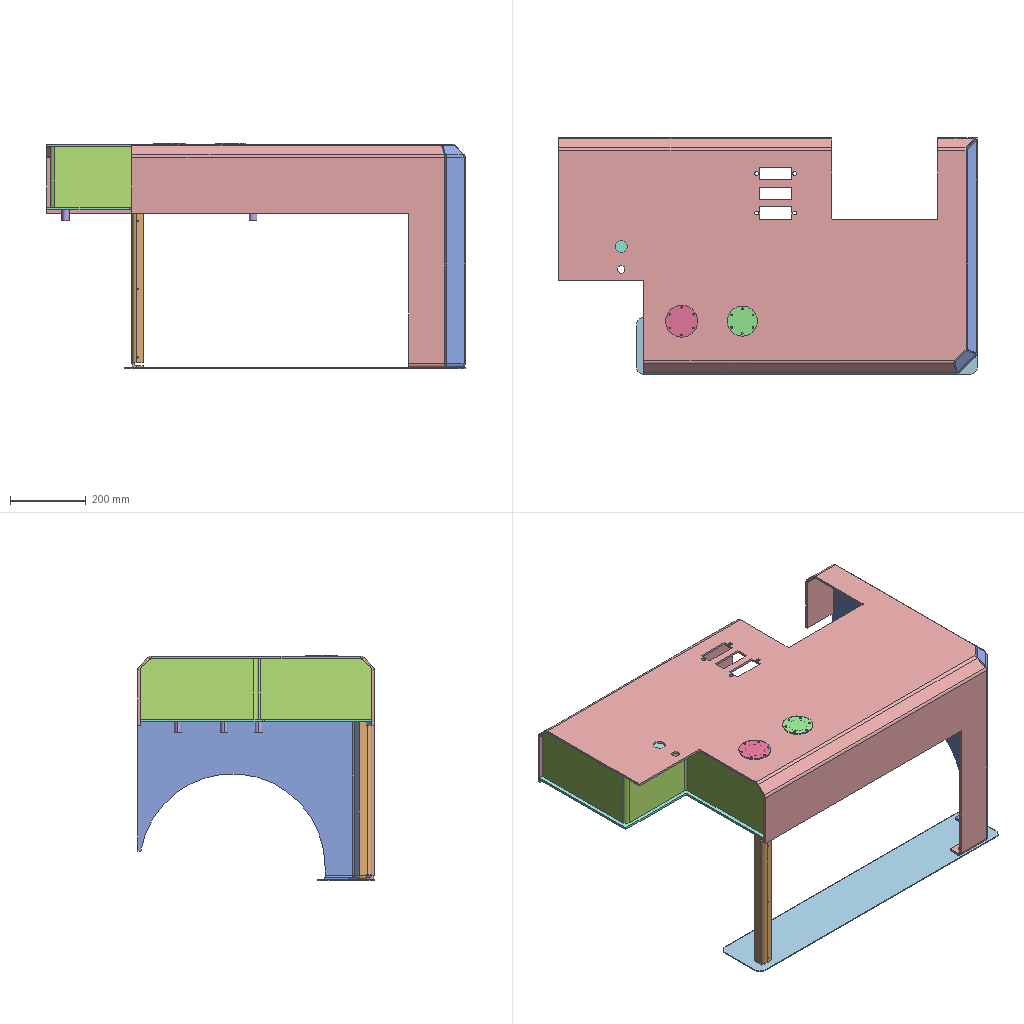Assembly | SolidWorks | 10 different items | 12 placed | box 1106 x 624 x 595 mm
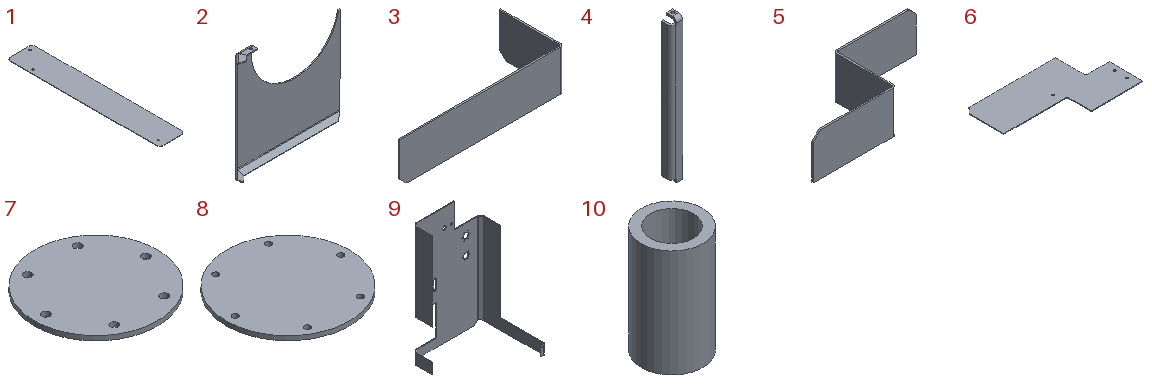Parts list (item | quantity | size | volume | features):
1 | x1 | 150 x 900 x 2.3 mm | 309143 mm3 | features FlatPattern 1, SMBaseFlange 1, SheetMetal 1
2 | x1 | 622 x 66.558 x 586.477 mm | 1620152 mm3 | features ICE 3, EdgeFlange 2, SMBaseFlange 2, Fillet 1, FlatPattern 1, SheetMetal 1
3 | x1 | 642 x 246 x 160 mm | 838612 mm3 | features Chamfer 1, Fillet 1, FlatPattern 1, SMBaseFlange 1, SheetMetal 1
4 | x1 | 34 x 30 x 418 mm | 132505 mm3 | features ICE 3, EdgeFlange 1, FlatPattern 1, SMBaseFlange 1, SheetMetal 1
5 | x1 | 612 x 231 x 160 mm | 791704 mm3 | features Chamfer 1, Fillet 1, FlatPattern 1, SMBaseFlange 1, SheetMetal 1
6 | x1 | 1100 x 612 x 6 mm | 2796793 mm3 | features Fillet 1, FlatPattern 1, SMBaseFlange 1, SheetMetal 1
7 | x1 | 80 x 80 x 3 mm | 14726 mm3 | features FlatPattern 1, SMBaseFlange 1, SheetMetal 1
8 | x1 | 85 x 85 x 3 mm | 16797 mm3 | features FlatPattern 1, SMBaseFlange 1, SheetMetal 1
9 | x1 | 624 x 590 x 1100 mm | 5059916 mm3 | features ICE 8, HoleWzd 2, Fillet 1, FlatPattern 1, SMBaseFlange 1, SheetMetal 1
10 | x3 | 20 x 20 x 35 mm | 5608 mm3 | features Extrusion 1
Mates (type | each side: item.copy, entity, surface, feature):
Coincident | 9.1 face plane Base-Flange1 | 2.1 face plane Base-Flange1
DistanceDim | 9.1 face plane Base-Flange1 | 2.1 face plane Base-Flange1
Coincident | 9.1 face plane Base-Flange1 | 2.1 face plane Edge-Flange2
Coincident | 9.1 face plane Base-Flange1 | 5.1 face plane Base-Flange1 | 2 times
DistanceDim | 9.1 face plane Cut-Extrude1 | 5.1 face plane Base-Flange1
Coincident | 2.1 face plane Base-Flange1 | 3.1 face plane Base-Flange1
Coincident | 9.1 face plane Base-Flange1 | 3.1 face plane Base-Flange1 | 2 times
Coincident | 5.1 face plane Base-Flange1 | 6.1 face plane Base-Flange1
Coincident | 9.1 face plane Base-Flange1 | 6.1 face plane Base-Flange1
Coincident | 2.1 face plane Base-Flange1 | 6.1 face plane Base-Flange1
Coincident | 6.1 face plane Base-Flange1 | 4.1 face plane Base-Flange1 | 2 times
Coincident | 9.1 face plane Base-Flange1 | 4.1 face plane Base-Flange1
Concentric | 6.1 face cylinder Base-Flange1 | 10.1 face cylinder Boss-Extrude1
DistanceDim | 10.1 face plane Boss-Extrude1 | 6.1 face plane Base-Flange1
Parallel | 10.1 plane | assembly plane
Concentric | 6.1 face cylinder Base-Flange1 | 10.2 face cylinder Boss-Extrude1
DistanceDim | 10.2 face plane Boss-Extrude1 | 6.1 face plane Base-Flange1
Parallel | 10.2 plane | assembly plane
Concentric | 6.1 face cylinder Base-Flange1 | 10.3 face cylinder Boss-Extrude1
DistanceDim | 10.3 face plane Boss-Extrude1 | 6.1 face plane Base-Flange1
Parallel | 10.3 plane | assembly plane
InPlace | 9.1 face plane Base-Flange1 | 7.1 plane
InPlace | 9.1 face plane Base-Flange1 | 8.1 plane
InPlace | 2.1 face plane Edge-Flange2 | 1.1 plane